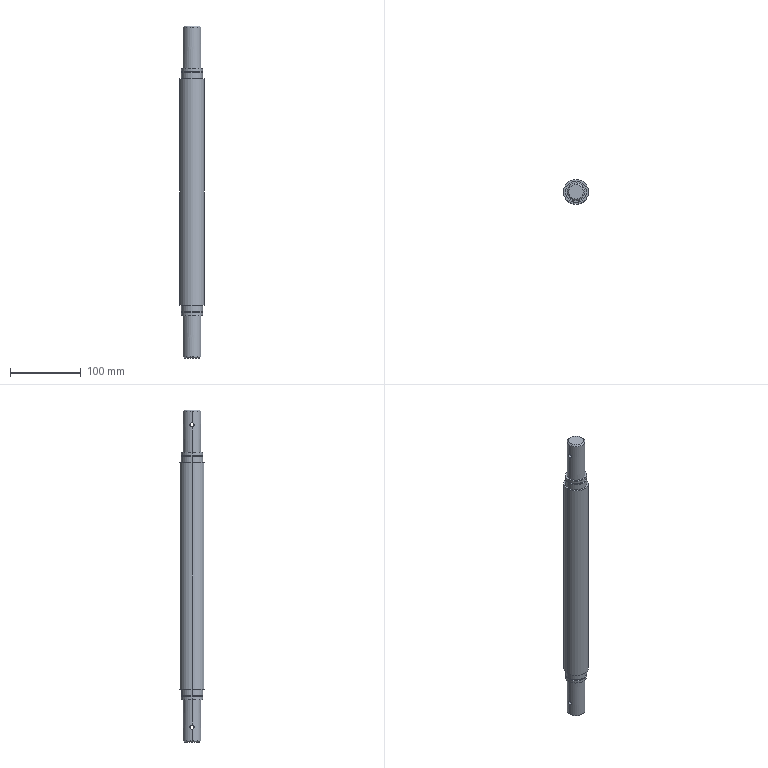Part | STEP file | Shaft 4 | 1 solid | 36 faces | box 35 x 35 x 470 mm | volume 385852 mm3 | cylinder 22 | plane 10 | cone 4 | commonest cylinder face diameters 30 x8 6 x4 25 x4 27.6 x4 35 x2
STEP:
#1=CARTESIAN_POINT('',(-17.5,0.,335.));
#2=VERTEX_POINT('',#1);
#3=CARTESIAN_POINT('',(17.5,0.,335.));
#4=VERTEX_POINT('',#3);
#5=CARTESIAN_POINT('',(0.,0.,335.));
#6=DIRECTION('',(0.,0.,-1.));
#7=DIRECTION('',(-1.,0.,0.));
#8=AXIS2_PLACEMENT_3D('',#5,#6,#7);
#9=CIRCLE('',#8,17.5);
#10=EDGE_CURVE('',#2,#4,#9,.T.);
#11=ORIENTED_EDGE('',*,*,#10,.T.);
#12=CARTESIAN_POINT('',(17.5,0.,15.));
#13=VERTEX_POINT('',#12);
#14=CARTESIAN_POINT('',(17.5,0.,350.));
#15=DIRECTION('',(0.,0.,-1.));
#16=VECTOR('',#15,1000.);
#17=LINE('',#14,#16);
#18=EDGE_CURVE('',#4,#13,#17,.T.);
#19=ORIENTED_EDGE('',*,*,#18,.T.);
#20=CARTESIAN_POINT('',(-17.5,0.,15.));
#21=VERTEX_POINT('',#20);
#22=CARTESIAN_POINT('',(0.,0.,15.));
#23=DIRECTION('',(0.,0.,1.));
#24=DIRECTION('',(-1.,0.,0.));
#25=AXIS2_PLACEMENT_3D('',#22,#23,#24);
#26=CIRCLE('',#25,17.5);
#27=EDGE_CURVE('',#13,#21,#26,.T.);
#28=ORIENTED_EDGE('',*,*,#27,.T.);
#29=CARTESIAN_POINT('',(-17.5,0.,350.));
#30=DIRECTION('',(0.,0.,-1.));
#31=VECTOR('',#30,1000.);
#32=LINE('',#29,#31);
#33=EDGE_CURVE('',#2,#21,#32,.T.);
#34=ORIENTED_EDGE('',*,*,#33,.F.);
#35=EDGE_LOOP('',(#11,#19,#28,#34));
#36=FACE_OUTER_BOUND('',#35,.T.);
#37=CARTESIAN_POINT('',(0.,0.,350.));
#38=DIRECTION('',(0.,0.,-1.));
#39=DIRECTION('',(-1.,0.,0.));
#40=AXIS2_PLACEMENT_3D('',#37,#38,#39);
#41=CYLINDRICAL_SURFACE('',#40,17.5);
#42=ADVANCED_FACE('',(#36),#41,.T.);
#43=CARTESIAN_POINT('',(15.,0.,15.));
#44=VERTEX_POINT('',#43);
#45=CARTESIAN_POINT('',(-15.,0.,15.));
#46=VERTEX_POINT('',#45);
#47=CARTESIAN_POINT('',(0.,0.,15.));
#48=DIRECTION('',(0.,0.,1.));
#49=DIRECTION('',(-1.,0.,0.));
#50=AXIS2_PLACEMENT_3D('',#47,#48,#49);
#51=CIRCLE('',#50,15.);
#52=EDGE_CURVE('',#44,#46,#51,.T.);
#53=ORIENTED_EDGE('',*,*,#52,.F.);
#54=CARTESIAN_POINT('',(15.,0.,6.));
#55=VERTEX_POINT('',#54);
#56=CARTESIAN_POINT('',(15.,0.,15.));
#57=DIRECTION('',(0.,0.,-1.));
#58=VECTOR('',#57,1000.);
#59=LINE('',#56,#58);
#60=EDGE_CURVE('',#44,#55,#59,.T.);
#61=ORIENTED_EDGE('',*,*,#60,.T.);
#62=CARTESIAN_POINT('',(-15.,0.,6.));
#63=VERTEX_POINT('',#62);
#64=CARTESIAN_POINT('',(0.,0.,6.));
#65=DIRECTION('',(0.,0.,1.));
#66=DIRECTION('',(-1.,0.,0.));
#67=AXIS2_PLACEMENT_3D('',#64,#65,#66);
#68=CIRCLE('',#67,15.);
#69=EDGE_CURVE('',#55,#63,#68,.T.);
#70=ORIENTED_EDGE('',*,*,#69,.T.);
#71=CARTESIAN_POINT('',(-15.,0.,15.));
#72=DIRECTION('',(0.,0.,-1.));
#73=VECTOR('',#72,1000.);
#74=LINE('',#71,#73);
#75=EDGE_CURVE('',#46,#63,#74,.T.);
#76=ORIENTED_EDGE('',*,*,#75,.F.);
#77=EDGE_LOOP('',(#53,#61,#70,#76));
#78=FACE_OUTER_BOUND('',#77,.T.);
#79=CARTESIAN_POINT('',(0.,0.,15.));
#80=DIRECTION('',(0.,0.,-1.));
#81=DIRECTION('',(-1.,0.,0.));
#82=AXIS2_PLACEMENT_3D('',#79,#80,#81);
#83=CYLINDRICAL_SURFACE('',#82,15.);
#84=ADVANCED_FACE('',(#78),#83,.T.);
#85=CARTESIAN_POINT('',(-15.,0.,335.));
#86=VERTEX_POINT('',#85);
#87=CARTESIAN_POINT('',(15.,0.,335.));
#88=VERTEX_POINT('',#87);
#89=CARTESIAN_POINT('',(0.,0.,335.));
#90=DIRECTION('',(0.,0.,-1.));
#91=DIRECTION('',(1.,0.,0.));
#92=AXIS2_PLACEMENT_3D('',#89,#90,#91);
#93=CIRCLE('',#92,15.);
#94=EDGE_CURVE('',#86,#88,#93,.T.);
#95=ORIENTED_EDGE('',*,*,#94,.F.);
#96=CARTESIAN_POINT('',(-15.,0.,344.));
#97=VERTEX_POINT('',#96);
#98=CARTESIAN_POINT('',(-15.,0.,335.));
#99=DIRECTION('',(0.,0.,1.));
#100=VECTOR('',#99,1000.);
#101=LINE('',#98,#100);
#102=EDGE_CURVE('',#86,#97,#101,.T.);
#103=ORIENTED_EDGE('',*,*,#102,.T.);
#104=CARTESIAN_POINT('',(15.,0.,344.));
#105=VERTEX_POINT('',#104);
#106=CARTESIAN_POINT('',(0.,0.,344.));
#107=DIRECTION('',(0.,0.,-1.));
#108=DIRECTION('',(1.,0.,0.));
#109=AXIS2_PLACEMENT_3D('',#106,#107,#108);
#110=CIRCLE('',#109,15.);
#111=EDGE_CURVE('',#97,#105,#110,.T.);
#112=ORIENTED_EDGE('',*,*,#111,.T.);
#113=CARTESIAN_POINT('',(15.,0.,335.));
#114=DIRECTION('',(0.,0.,1.));
#115=VECTOR('',#114,1000.);
#116=LINE('',#113,#115);
#117=EDGE_CURVE('',#88,#105,#116,.T.);
#118=ORIENTED_EDGE('',*,*,#117,.F.);
#119=EDGE_LOOP('',(#95,#103,#112,#118));
#120=FACE_OUTER_BOUND('',#119,.T.);
#121=CARTESIAN_POINT('',(0.,0.,335.));
#122=DIRECTION('',(0.,0.,1.));
#123=DIRECTION('',(1.,0.,0.));
#124=AXIS2_PLACEMENT_3D('',#121,#122,#123);
#125=CYLINDRICAL_SURFACE('',#124,15.);
#126=ADVANCED_FACE('',(#120),#125,.T.);
#127=CARTESIAN_POINT('',(-13.8,0.,6.));
#128=VERTEX_POINT('',#127);
#129=CARTESIAN_POINT('',(13.8,0.,6.));
#130=VERTEX_POINT('',#129);
#131=CARTESIAN_POINT('',(0.,0.,6.));
#132=DIRECTION('',(0.,0.,-1.));
#133=DIRECTION('',(-1.,0.,0.));
#134=AXIS2_PLACEMENT_3D('',#131,#132,#133);
#135=CIRCLE('',#134,13.8);
#136=EDGE_CURVE('',#128,#130,#135,.T.);
#137=ORIENTED_EDGE('',*,*,#136,.T.);
#138=CARTESIAN_POINT('',(13.8,0.,4.));
#139=VERTEX_POINT('',#138);
#140=CARTESIAN_POINT('',(13.8,0.,0.));
#141=DIRECTION('',(0.,0.,-1.));
#142=VECTOR('',#141,1000.);
#143=LINE('',#140,#142);
#144=EDGE_CURVE('',#130,#139,#143,.T.);
#145=ORIENTED_EDGE('',*,*,#144,.T.);
#146=CARTESIAN_POINT('',(-13.8,0.,4.));
#147=VERTEX_POINT('',#146);
#148=CARTESIAN_POINT('',(0.,0.,4.));
#149=DIRECTION('',(0.,0.,1.));
#150=DIRECTION('',(-1.,0.,0.));
#151=AXIS2_PLACEMENT_3D('',#148,#149,#150);
#152=CIRCLE('',#151,13.8);
#153=EDGE_CURVE('',#139,#147,#152,.T.);
#154=ORIENTED_EDGE('',*,*,#153,.T.);
#155=CARTESIAN_POINT('',(-13.8,0.,0.));
#156=DIRECTION('',(0.,0.,-1.));
#157=VECTOR('',#156,1000.);
#158=LINE('',#155,#157);
#159=EDGE_CURVE('',#128,#147,#158,.T.);
#160=ORIENTED_EDGE('',*,*,#159,.F.);
#161=EDGE_LOOP('',(#137,#145,#154,#160));
#162=FACE_OUTER_BOUND('',#161,.T.);
#163=CARTESIAN_POINT('',(0.,0.,0.));
#164=DIRECTION('',(0.,0.,-1.));
#165=DIRECTION('',(-1.,0.,0.));
#166=AXIS2_PLACEMENT_3D('',#163,#164,#165);
#167=CYLINDRICAL_SURFACE('',#166,13.8);
#168=ADVANCED_FACE('',(#162),#167,.T.);
#169=CARTESIAN_POINT('',(-13.8,0.,346.));
#170=VERTEX_POINT('',#169);
#171=CARTESIAN_POINT('',(13.8,0.,346.));
#172=VERTEX_POINT('',#171);
#173=CARTESIAN_POINT('',(0.,0.,346.));
#174=DIRECTION('',(0.,0.,-1.));
#175=DIRECTION('',(-1.,0.,0.));
#176=AXIS2_PLACEMENT_3D('',#173,#174,#175);
#177=CIRCLE('',#176,13.8);
#178=EDGE_CURVE('',#170,#172,#177,.T.);
#179=ORIENTED_EDGE('',*,*,#178,.T.);
#180=CARTESIAN_POINT('',(13.8,0.,344.));
#181=VERTEX_POINT('',#180);
#182=CARTESIAN_POINT('',(13.8,0.,0.));
#183=DIRECTION('',(0.,0.,-1.));
#184=VECTOR('',#183,1000.);
#185=LINE('',#182,#184);
#186=EDGE_CURVE('',#172,#181,#185,.T.);
#187=ORIENTED_EDGE('',*,*,#186,.T.);
#188=CARTESIAN_POINT('',(-13.8,0.,344.));
#189=VERTEX_POINT('',#188);
#190=CARTESIAN_POINT('',(0.,0.,344.));
#191=DIRECTION('',(0.,0.,1.));
#192=DIRECTION('',(-1.,0.,0.));
#193=AXIS2_PLACEMENT_3D('',#190,#191,#192);
#194=CIRCLE('',#193,13.8);
#195=EDGE_CURVE('',#181,#189,#194,.T.);
#196=ORIENTED_EDGE('',*,*,#195,.T.);
#197=CARTESIAN_POINT('',(-13.8,0.,0.));
#198=DIRECTION('',(0.,0.,-1.));
#199=VECTOR('',#198,1000.);
#200=LINE('',#197,#199);
#201=EDGE_CURVE('',#170,#189,#200,.T.);
#202=ORIENTED_EDGE('',*,*,#201,.F.);
#203=EDGE_LOOP('',(#179,#187,#196,#202));
#204=FACE_OUTER_BOUND('',#203,.T.);
#205=CARTESIAN_POINT('',(0.,0.,0.));
#206=DIRECTION('',(0.,0.,-1.));
#207=DIRECTION('',(-1.,0.,0.));
#208=AXIS2_PLACEMENT_3D('',#205,#206,#207);
#209=CYLINDRICAL_SURFACE('',#208,13.8);
#210=ADVANCED_FACE('',(#204),#209,.T.);
#211=CARTESIAN_POINT('',(-15.,0.,4.));
#212=VERTEX_POINT('',#211);
#213=CARTESIAN_POINT('',(15.,0.,4.));
#214=VERTEX_POINT('',#213);
#215=CARTESIAN_POINT('',(0.,0.,4.));
#216=DIRECTION('',(0.,0.,-1.));
#217=DIRECTION('',(-1.,0.,0.));
#218=AXIS2_PLACEMENT_3D('',#215,#216,#217);
#219=CIRCLE('',#218,15.);
#220=EDGE_CURVE('',#212,#214,#219,.T.);
#221=ORIENTED_EDGE('',*,*,#220,.T.);
#222=CARTESIAN_POINT('',(15.,0.,0.));
#223=VERTEX_POINT('',#222);
#224=CARTESIAN_POINT('',(15.,0.,15.));
#225=DIRECTION('',(0.,0.,-1.));
#226=VECTOR('',#225,1000.);
#227=LINE('',#224,#226);
#228=EDGE_CURVE('',#214,#223,#227,.T.);
#229=ORIENTED_EDGE('',*,*,#228,.T.);
#230=CARTESIAN_POINT('',(-15.,0.,0.));
#231=VERTEX_POINT('',#230);
#232=CARTESIAN_POINT('',(0.,0.,0.));
#233=DIRECTION('',(0.,0.,1.));
#234=DIRECTION('',(-1.,0.,0.));
#235=AXIS2_PLACEMENT_3D('',#232,#233,#234);
#236=CIRCLE('',#235,15.);
#237=EDGE_CURVE('',#223,#231,#236,.T.);
#238=ORIENTED_EDGE('',*,*,#237,.T.);
#239=CARTESIAN_POINT('',(-15.,0.,15.));
#240=DIRECTION('',(0.,0.,-1.));
#241=VECTOR('',#240,1000.);
#242=LINE('',#239,#241);
#243=EDGE_CURVE('',#212,#231,#242,.T.);
#244=ORIENTED_EDGE('',*,*,#243,.F.);
#245=EDGE_LOOP('',(#221,#229,#238,#244));
#246=FACE_OUTER_BOUND('',#245,.T.);
#247=CARTESIAN_POINT('',(0.,0.,15.));
#248=DIRECTION('',(0.,0.,-1.));
#249=DIRECTION('',(-1.,0.,0.));
#250=AXIS2_PLACEMENT_3D('',#247,#248,#249);
#251=CYLINDRICAL_SURFACE('',#250,15.);
#252=ADVANCED_FACE('',(#246),#251,.T.);
#253=CARTESIAN_POINT('',(15.,0.,346.));
#254=VERTEX_POINT('',#253);
#255=CARTESIAN_POINT('',(-15.,0.,346.));
#256=VERTEX_POINT('',#255);
#257=CARTESIAN_POINT('',(0.,0.,346.));
#258=DIRECTION('',(0.,0.,1.));
#259=DIRECTION('',(1.,0.,0.));
#260=AXIS2_PLACEMENT_3D('',#257,#258,#259);
#261=CIRCLE('',#260,15.);
#262=EDGE_CURVE('',#254,#256,#261,.T.);
#263=ORIENTED_EDGE('',*,*,#262,.T.);
#264=CARTESIAN_POINT('',(-15.,0.,350.));
#265=VERTEX_POINT('',#264);
#266=CARTESIAN_POINT('',(-15.,0.,335.));
#267=DIRECTION('',(0.,0.,1.));
#268=VECTOR('',#267,1000.);
#269=LINE('',#266,#268);
#270=EDGE_CURVE('',#256,#265,#269,.T.);
#271=ORIENTED_EDGE('',*,*,#270,.T.);
#272=CARTESIAN_POINT('',(15.,0.,350.));
#273=VERTEX_POINT('',#272);
#274=CARTESIAN_POINT('',(0.,0.,350.));
#275=DIRECTION('',(0.,0.,-1.));
#276=DIRECTION('',(1.,0.,0.));
#277=AXIS2_PLACEMENT_3D('',#274,#275,#276);
#278=CIRCLE('',#277,15.);
#279=EDGE_CURVE('',#265,#273,#278,.T.);
#280=ORIENTED_EDGE('',*,*,#279,.T.);
#281=CARTESIAN_POINT('',(15.,0.,335.));
#282=DIRECTION('',(0.,0.,1.));
#283=VECTOR('',#282,1000.);
#284=LINE('',#281,#283);
#285=EDGE_CURVE('',#254,#273,#284,.T.);
#286=ORIENTED_EDGE('',*,*,#285,.F.);
#287=EDGE_LOOP('',(#263,#271,#280,#286));
#288=FACE_OUTER_BOUND('',#287,.T.);
#289=CARTESIAN_POINT('',(0.,0.,335.));
#290=DIRECTION('',(0.,0.,1.));
#291=DIRECTION('',(1.,0.,0.));
#292=AXIS2_PLACEMENT_3D('',#289,#290,#291);
#293=CYLINDRICAL_SURFACE('',#292,15.);
#294=ADVANCED_FACE('',(#288),#293,.T.);
#295=CARTESIAN_POINT('',(0.,12.5,-58.));
#296=VERTEX_POINT('',#295);
#297=CARTESIAN_POINT('',(-12.5,0.,-58.));
#298=VERTEX_POINT('',#297);
#299=CARTESIAN_POINT('',(0.,0.,-58.));
#300=DIRECTION('',(0.,0.,1.));
#301=DIRECTION('',(1.,0.,0.));
#302=AXIS2_PLACEMENT_3D('',#299,#300,#301);
#303=CIRCLE('',#302,12.5);
#304=EDGE_CURVE('',#296,#298,#303,.T.);
#305=ORIENTED_EDGE('',*,*,#304,.T.);
#306=CARTESIAN_POINT('',(-12.5,0.,-42.));
#307=VERTEX_POINT('',#306);
#308=CARTESIAN_POINT('',(-12.5,0.,-60.));
#309=DIRECTION('',(0.,0.,1.));
#310=VECTOR('',#309,1000.);
#311=LINE('',#308,#310);
#312=EDGE_CURVE('',#298,#307,#311,.T.);
#313=ORIENTED_EDGE('',*,*,#312,.T.);
#314=CARTESIAN_POINT('',(-12.5,0.,-36.));
#315=VERTEX_POINT('',#314);
#316=CARTESIAN_POINT('',(-12.5,0.,-42.));
#317=CARTESIAN_POINT('',(-12.5,0.1989,-42.));
#318=CARTESIAN_POINT('',(-12.495,0.3944,-41.98));
#319=CARTESIAN_POINT('',(-12.477,0.7788,-41.904));
#320=CARTESIAN_POINT('',(-12.464,0.9697,-41.846));
#321=CARTESIAN_POINT('',(-12.43,1.333,-41.695));
#322=CARTESIAN_POINT('',(-12.41,1.505,-41.603));
#323=CARTESIAN_POINT('',(-12.366,1.83,-41.385));
#324=CARTESIAN_POINT('',(-12.342,1.984,-41.259));
#325=CARTESIAN_POINT('',(-12.295,2.259,-40.983));
#326=CARTESIAN_POINT('',(-12.271,2.383,-40.833));
#327=CARTESIAN_POINT('',(-12.227,2.602,-40.505));
#328=CARTESIAN_POINT('',(-12.206,2.695,-40.332));
#329=CARTESIAN_POINT('',(-12.172,2.845,-39.971));
#330=CARTESIAN_POINT('',(-12.158,2.903,-39.782));
#331=CARTESIAN_POINT('',(-12.14,2.981,-39.394));
#332=CARTESIAN_POINT('',(-12.135,3.,-39.199));
#333=CARTESIAN_POINT('',(-12.135,3.,-38.806));
#334=CARTESIAN_POINT('',(-12.14,2.981,-38.607));
#335=CARTESIAN_POINT('',(-12.158,2.904,-38.221));
#336=CARTESIAN_POINT('',(-12.172,2.847,-38.034));
#337=CARTESIAN_POINT('',(-12.206,2.696,-37.67));
#338=CARTESIAN_POINT('',(-12.227,2.603,-37.495));
#339=CARTESIAN_POINT('',(-12.271,2.386,-37.171));
#340=CARTESIAN_POINT('',(-12.295,2.261,-37.019));
#341=CARTESIAN_POINT('',(-12.342,1.983,-36.741));
#342=CARTESIAN_POINT('',(-12.366,1.833,-36.617));
#343=CARTESIAN_POINT('',(-12.41,1.509,-36.4));
#344=CARTESIAN_POINT('',(-12.43,1.333,-36.305));
#345=CARTESIAN_POINT('',(-12.464,0.9711,-36.155));
#346=CARTESIAN_POINT('',(-12.477,0.7841,-36.098));
#347=CARTESIAN_POINT('',(-12.495,0.3981,-36.02));
#348=CARTESIAN_POINT('',(-12.5,0.1989,-36.));
#349=CARTESIAN_POINT('',(-12.5,0.,-36.));
#350=B_SPLINE_CURVE_WITH_KNOTS('',3,(#316,#317,#318,#319,#320,#321,#322,#323,#324,#325,#326,#327,#328,#329,#330,#331,#332,#333,#334,#335,#336,#337,#338,#339,#340,#341,#342,#343,#344,#345,#346,#347,#348,#349),.UNSPECIFIED.,.F.,.F.,(4,2,2,2,2,2,2,2,2,2,2,2,2,2,2,2,4),(0.009411,0.009999,0.01059,0.01118,0.01176,0.01235,0.01294,0.01353,0.01412,0.0147,0.01529,0.01588,0.01647,0.01706,0.01765,0.01823,0.01882),.UNSPECIFIED.);
#351=EDGE_CURVE('',#307,#315,#350,.T.);
#352=ORIENTED_EDGE('',*,*,#351,.T.);
#353=CARTESIAN_POINT('',(-12.5,0.,0.));
#354=VERTEX_POINT('',#353);
#355=CARTESIAN_POINT('',(-12.5,0.,-60.));
#356=DIRECTION('',(0.,0.,1.));
#357=VECTOR('',#356,1000.);
#358=LINE('',#355,#357);
#359=EDGE_CURVE('',#315,#354,#358,.T.);
#360=ORIENTED_EDGE('',*,*,#359,.T.);
#361=CARTESIAN_POINT('',(12.5,0.,0.));
#362=VERTEX_POINT('',#361);
#363=CARTESIAN_POINT('',(0.,0.,0.));
#364=DIRECTION('',(0.,0.,-1.));
#365=DIRECTION('',(1.,0.,0.));
#366=AXIS2_PLACEMENT_3D('',#363,#364,#365);
#367=CIRCLE('',#366,12.5);
#368=EDGE_CURVE('',#354,#362,#367,.T.);
#369=ORIENTED_EDGE('',*,*,#368,.T.);
#370=CARTESIAN_POINT('',(12.5,0.,-36.));
#371=VERTEX_POINT('',#370);
#372=CARTESIAN_POINT('',(12.5,0.,-60.));
#373=DIRECTION('',(0.,0.,1.));
#374=VECTOR('',#373,1000.);
#375=LINE('',#372,#374);
#376=EDGE_CURVE('',#371,#362,#375,.T.);
#377=ORIENTED_EDGE('',*,*,#376,.F.);
#378=CARTESIAN_POINT('',(12.5,0.,-42.));
#379=VERTEX_POINT('',#378);
#380=CARTESIAN_POINT('',(12.5,0.,-36.));
#381=CARTESIAN_POINT('',(12.5,0.1989,-36.));
#382=CARTESIAN_POINT('',(12.495,0.3944,-36.02));
#383=CARTESIAN_POINT('',(12.477,0.7788,-36.096));
#384=CARTESIAN_POINT('',(12.464,0.9697,-36.154));
#385=CARTESIAN_POINT('',(12.43,1.333,-36.305));
#386=CARTESIAN_POINT('',(12.41,1.505,-36.397));
#387=CARTESIAN_POINT('',(12.366,1.83,-36.615));
#388=CARTESIAN_POINT('',(12.342,1.984,-36.741));
#389=CARTESIAN_POINT('',(12.295,2.259,-37.017));
#390=CARTESIAN_POINT('',(12.271,2.383,-37.167));
#391=CARTESIAN_POINT('',(12.227,2.602,-37.495));
#392=CARTESIAN_POINT('',(12.206,2.695,-37.668));
#393=CARTESIAN_POINT('',(12.172,2.845,-38.029));
#394=CARTESIAN_POINT('',(12.158,2.903,-38.218));
#395=CARTESIAN_POINT('',(12.14,2.981,-38.606));
#396=CARTESIAN_POINT('',(12.135,3.,-38.801));
#397=CARTESIAN_POINT('',(12.135,3.,-39.194));
#398=CARTESIAN_POINT('',(12.14,2.981,-39.393));
#399=CARTESIAN_POINT('',(12.158,2.904,-39.779));
#400=CARTESIAN_POINT('',(12.172,2.847,-39.966));
#401=CARTESIAN_POINT('',(12.206,2.696,-40.33));
#402=CARTESIAN_POINT('',(12.227,2.603,-40.505));
#403=CARTESIAN_POINT('',(12.271,2.386,-40.829));
#404=CARTESIAN_POINT('',(12.295,2.261,-40.981));
#405=CARTESIAN_POINT('',(12.342,1.983,-41.259));
#406=CARTESIAN_POINT('',(12.366,1.833,-41.383));
#407=CARTESIAN_POINT('',(12.41,1.509,-41.6));
#408=CARTESIAN_POINT('',(12.43,1.333,-41.695));
#409=CARTESIAN_POINT('',(12.464,0.9711,-41.845));
#410=CARTESIAN_POINT('',(12.477,0.7841,-41.902));
#411=CARTESIAN_POINT('',(12.495,0.3981,-41.98));
#412=CARTESIAN_POINT('',(12.5,0.1989,-42.));
#413=CARTESIAN_POINT('',(12.5,0.,-42.));
#414=B_SPLINE_CURVE_WITH_KNOTS('',3,(#380,#381,#382,#383,#384,#385,#386,#387,#388,#389,#390,#391,#392,#393,#394,#395,#396,#397,#398,#399,#400,#401,#402,#403,#404,#405,#406,#407,#408,#409,#410,#411,#412,#413),.UNSPECIFIED.,.F.,.F.,(4,2,2,2,2,2,2,2,2,2,2,2,2,2,2,2,4),(0.009411,0.009999,0.01059,0.01118,0.01176,0.01235,0.01294,0.01353,0.01412,0.0147,0.01529,0.01588,0.01647,0.01706,0.01765,0.01823,0.01882),.UNSPECIFIED.);
#415=EDGE_CURVE('',#371,#379,#414,.T.);
#416=ORIENTED_EDGE('',*,*,#415,.T.);
#417=CARTESIAN_POINT('',(12.5,0.,-58.));
#418=VERTEX_POINT('',#417);
#419=CARTESIAN_POINT('',(12.5,0.,-60.));
#420=DIRECTION('',(0.,0.,1.));
#421=VECTOR('',#420,1000.);
#422=LINE('',#419,#421);
#423=EDGE_CURVE('',#418,#379,#422,.T.);
#424=ORIENTED_EDGE('',*,*,#423,.F.);
#425=CARTESIAN_POINT('',(0.,0.,-58.));
#426=DIRECTION('',(0.,0.,1.));
#427=DIRECTION('',(1.,0.,0.));
#428=AXIS2_PLACEMENT_3D('',#425,#426,#427);
#429=CIRCLE('',#428,12.5);
#430=EDGE_CURVE('',#418,#296,#429,.T.);
#431=ORIENTED_EDGE('',*,*,#430,.T.);
#432=EDGE_LOOP('',(#305,#313,#352,#360,#369,#377,#416,#424,#431));
#433=FACE_OUTER_BOUND('',#432,.T.);
#434=CARTESIAN_POINT('',(0.,0.,-60.));
#435=DIRECTION('',(0.,0.,1.));
#436=DIRECTION('',(1.,0.,0.));
#437=AXIS2_PLACEMENT_3D('',#434,#435,#436);
#438=CYLINDRICAL_SURFACE('',#437,12.5);
#439=ADVANCED_FACE('',(#433),#438,.T.);
#440=CARTESIAN_POINT('',(0.,12.5,408.));
#441=VERTEX_POINT('',#440);
#442=CARTESIAN_POINT('',(12.5,0.,408.));
#443=VERTEX_POINT('',#442);
#444=CARTESIAN_POINT('',(0.,0.,408.));
#445=DIRECTION('',(0.,0.,-1.));
#446=DIRECTION('',(-1.,0.,0.));
#447=AXIS2_PLACEMENT_3D('',#444,#445,#446);
#448=CIRCLE('',#447,12.5);
#449=EDGE_CURVE('',#441,#443,#448,.T.);
#450=ORIENTED_EDGE('',*,*,#449,.T.);
#451=CARTESIAN_POINT('',(12.5,0.,392.));
#452=VERTEX_POINT('',#451);
#453=CARTESIAN_POINT('',(12.5,0.,410.));
#454=DIRECTION('',(0.,0.,-1.));
#455=VECTOR('',#454,1000.);
#456=LINE('',#453,#455);
#457=EDGE_CURVE('',#443,#452,#456,.T.);
#458=ORIENTED_EDGE('',*,*,#457,.T.);
#459=CARTESIAN_POINT('',(12.5,0.,386.));
#460=VERTEX_POINT('',#459);
#461=CARTESIAN_POINT('',(12.5,0.,392.));
#462=CARTESIAN_POINT('',(12.5,0.1989,392.));
#463=CARTESIAN_POINT('',(12.495,0.3944,391.98));
#464=CARTESIAN_POINT('',(12.477,0.7788,391.904));
#465=CARTESIAN_POINT('',(12.464,0.9697,391.846));
#466=CARTESIAN_POINT('',(12.43,1.333,391.695));
#467=CARTESIAN_POINT('',(12.41,1.505,391.603));
#468=CARTESIAN_POINT('',(12.366,1.83,391.385));
#469=CARTESIAN_POINT('',(12.342,1.984,391.259));
#470=CARTESIAN_POINT('',(12.295,2.259,390.983));
#471=CARTESIAN_POINT('',(12.271,2.383,390.833));
#472=CARTESIAN_POINT('',(12.227,2.602,390.505));
#473=CARTESIAN_POINT('',(12.206,2.695,390.332));
#474=CARTESIAN_POINT('',(12.172,2.845,389.971));
#475=CARTESIAN_POINT('',(12.158,2.903,389.782));
#476=CARTESIAN_POINT('',(12.14,2.981,389.394));
#477=CARTESIAN_POINT('',(12.135,3.,389.199));
#478=CARTESIAN_POINT('',(12.135,3.,388.806));
#479=CARTESIAN_POINT('',(12.14,2.981,388.607));
#480=CARTESIAN_POINT('',(12.158,2.904,388.221));
#481=CARTESIAN_POINT('',(12.172,2.847,388.034));
#482=CARTESIAN_POINT('',(12.206,2.696,387.67));
#483=CARTESIAN_POINT('',(12.227,2.603,387.495));
#484=CARTESIAN_POINT('',(12.271,2.386,387.171));
#485=CARTESIAN_POINT('',(12.295,2.261,387.019));
#486=CARTESIAN_POINT('',(12.342,1.983,386.741));
#487=CARTESIAN_POINT('',(12.366,1.833,386.617));
#488=CARTESIAN_POINT('',(12.41,1.509,386.4));
#489=CARTESIAN_POINT('',(12.43,1.333,386.305));
#490=CARTESIAN_POINT('',(12.464,0.9711,386.155));
#491=CARTESIAN_POINT('',(12.477,0.7841,386.098));
#492=CARTESIAN_POINT('',(12.495,0.3981,386.02));
#493=CARTESIAN_POINT('',(12.5,0.1989,386.));
#494=CARTESIAN_POINT('',(12.5,0.,386.));
#495=B_SPLINE_CURVE_WITH_KNOTS('',3,(#461,#462,#463,#464,#465,#466,#467,#468,#469,#470,#471,#472,#473,#474,#475,#476,#477,#478,#479,#480,#481,#482,#483,#484,#485,#486,#487,#488,#489,#490,#491,#492,#493,#494),.UNSPECIFIED.,.F.,.F.,(4,2,2,2,2,2,2,2,2,2,2,2,2,2,2,2,4),(0.,0.0005882,0.001176,0.001765,0.002353,0.002941,0.003529,0.004117,0.004706,0.005294,0.005882,0.00647,0.007058,0.007646,0.008235,0.008823,0.009411),.UNSPECIFIED.);
#496=EDGE_CURVE('',#452,#460,#495,.T.);
#497=ORIENTED_EDGE('',*,*,#496,.T.);
#498=CARTESIAN_POINT('',(12.5,0.,350.));
#499=VERTEX_POINT('',#498);
#500=CARTESIAN_POINT('',(12.5,0.,410.));
#501=DIRECTION('',(0.,0.,-1.));
#502=VECTOR('',#501,1000.);
#503=LINE('',#500,#502);
#504=EDGE_CURVE('',#460,#499,#503,.T.);
#505=ORIENTED_EDGE('',*,*,#504,.T.);
#506=CARTESIAN_POINT('',(-12.5,0.,350.));
#507=VERTEX_POINT('',#506);
#508=CARTESIAN_POINT('',(0.,0.,350.));
#509=DIRECTION('',(0.,0.,-1.));
#510=DIRECTION('',(-1.,0.,0.));
#511=AXIS2_PLACEMENT_3D('',#508,#509,#510);
#512=CIRCLE('',#511,12.5);
#513=EDGE_CURVE('',#507,#499,#512,.T.);
#514=ORIENTED_EDGE('',*,*,#513,.F.);
#515=CARTESIAN_POINT('',(-12.5,0.,386.));
#516=VERTEX_POINT('',#515);
#517=CARTESIAN_POINT('',(-12.5,0.,410.));
#518=DIRECTION('',(0.,0.,-1.));
#519=VECTOR('',#518,1000.);
#520=LINE('',#517,#519);
#521=EDGE_CURVE('',#516,#507,#520,.T.);
#522=ORIENTED_EDGE('',*,*,#521,.F.);
#523=CARTESIAN_POINT('',(-12.5,0.,392.));
#524=VERTEX_POINT('',#523);
#525=CARTESIAN_POINT('',(-12.5,0.,386.));
#526=CARTESIAN_POINT('',(-12.5,0.1989,386.));
#527=CARTESIAN_POINT('',(-12.495,0.3944,386.02));
#528=CARTESIAN_POINT('',(-12.477,0.7788,386.096));
#529=CARTESIAN_POINT('',(-12.464,0.9697,386.154));
#530=CARTESIAN_POINT('',(-12.43,1.333,386.305));
#531=CARTESIAN_POINT('',(-12.41,1.505,386.397));
#532=CARTESIAN_POINT('',(-12.366,1.83,386.615));
#533=CARTESIAN_POINT('',(-12.342,1.984,386.741));
#534=CARTESIAN_POINT('',(-12.295,2.259,387.017));
#535=CARTESIAN_POINT('',(-12.271,2.383,387.167));
#536=CARTESIAN_POINT('',(-12.227,2.602,387.495));
#537=CARTESIAN_POINT('',(-12.206,2.695,387.668));
#538=CARTESIAN_POINT('',(-12.172,2.845,388.029));
#539=CARTESIAN_POINT('',(-12.158,2.903,388.218));
#540=CARTESIAN_POINT('',(-12.14,2.981,388.606));
#541=CARTESIAN_POINT('',(-12.135,3.,388.801));
#542=CARTESIAN_POINT('',(-12.135,3.,389.194));
#543=CARTESIAN_POINT('',(-12.14,2.981,389.393));
#544=CARTESIAN_POINT('',(-12.158,2.904,389.779));
#545=CARTESIAN_POINT('',(-12.172,2.847,389.966));
#546=CARTESIAN_POINT('',(-12.206,2.696,390.33));
#547=CARTESIAN_POINT('',(-12.227,2.603,390.505));
#548=CARTESIAN_POINT('',(-12.271,2.386,390.829));
#549=CARTESIAN_POINT('',(-12.295,2.261,390.981));
#550=CARTESIAN_POINT('',(-12.342,1.983,391.259));
#551=CARTESIAN_POINT('',(-12.366,1.833,391.383));
#552=CARTESIAN_POINT('',(-12.41,1.509,391.6));
#553=CARTESIAN_POINT('',(-12.43,1.333,391.695));
#554=CARTESIAN_POINT('',(-12.464,0.9711,391.845));
#555=CARTESIAN_POINT('',(-12.477,0.7841,391.902));
#556=CARTESIAN_POINT('',(-12.495,0.3981,391.98));
#557=CARTESIAN_POINT('',(-12.5,0.1989,392.));
#558=CARTESIAN_POINT('',(-12.5,0.,392.));
#559=B_SPLINE_CURVE_WITH_KNOTS('',3,(#525,#526,#527,#528,#529,#530,#531,#532,#533,#534,#535,#536,#537,#538,#539,#540,#541,#542,#543,#544,#545,#546,#547,#548,#549,#550,#551,#552,#553,#554,#555,#556,#557,#558),.UNSPECIFIED.,.F.,.F.,(4,2,2,2,2,2,2,2,2,2,2,2,2,2,2,2,4),(0.,0.0005882,0.001176,0.001765,0.002353,0.002941,0.003529,0.004117,0.004706,0.005294,0.005882,0.00647,0.007058,0.007646,0.008235,0.008823,0.009411),.UNSPECIFIED.);
#560=EDGE_CURVE('',#516,#524,#559,.T.);
#561=ORIENTED_EDGE('',*,*,#560,.T.);
#562=CARTESIAN_POINT('',(-12.5,0.,408.));
#563=VERTEX_POINT('',#562);
#564=CARTESIAN_POINT('',(-12.5,0.,410.));
#565=DIRECTION('',(0.,0.,-1.));
#566=VECTOR('',#565,1000.);
#567=LINE('',#564,#566);
#568=EDGE_CURVE('',#563,#524,#567,.T.);
#569=ORIENTED_EDGE('',*,*,#568,.F.);
#570=CARTESIAN_POINT('',(0.,0.,408.));
#571=DIRECTION('',(0.,0.,-1.));
#572=DIRECTION('',(-1.,0.,0.));
#573=AXIS2_PLACEMENT_3D('',#570,#571,#572);
#574=CIRCLE('',#573,12.5);
#575=EDGE_CURVE('',#563,#441,#574,.T.);
#576=ORIENTED_EDGE('',*,*,#575,.T.);
#577=EDGE_LOOP('',(#450,#458,#497,#505,#514,#522,#561,#569,#576));
#578=FACE_OUTER_BOUND('',#577,.T.);
#579=CARTESIAN_POINT('',(0.,0.,410.));
#580=DIRECTION('',(0.,0.,-1.));
#581=DIRECTION('',(-1.,0.,0.));
#582=AXIS2_PLACEMENT_3D('',#579,#580,#581);
#583=CYLINDRICAL_SURFACE('',#582,12.5);
#584=ADVANCED_FACE('',(#578),#583,.T.);
#585=CARTESIAN_POINT('',(-12.5,0.,-36.));
#586=CARTESIAN_POINT('',(-12.5,-0.1989,-36.));
#587=CARTESIAN_POINT('',(-12.495,-0.3944,-36.02));
#588=CARTESIAN_POINT('',(-12.477,-0.7788,-36.096));
#589=CARTESIAN_POINT('',(-12.464,-0.9697,-36.154));
#590=CARTESIAN_POINT('',(-12.43,-1.333,-36.305));
#591=CARTESIAN_POINT('',(-12.41,-1.505,-36.397));
#592=CARTESIAN_POINT('',(-12.366,-1.83,-36.615));
#593=CARTESIAN_POINT('',(-12.342,-1.984,-36.741));
#594=CARTESIAN_POINT('',(-12.295,-2.259,-37.017));
#595=CARTESIAN_POINT('',(-12.271,-2.383,-37.167));
#596=CARTESIAN_POINT('',(-12.227,-2.602,-37.495));
#597=CARTESIAN_POINT('',(-12.206,-2.695,-37.668));
#598=CARTESIAN_POINT('',(-12.172,-2.845,-38.029));
#599=CARTESIAN_POINT('',(-12.158,-2.903,-38.218));
#600=CARTESIAN_POINT('',(-12.14,-2.981,-38.606));
#601=CARTESIAN_POINT('',(-12.135,-3.,-38.801));
#602=CARTESIAN_POINT('',(-12.135,-3.,-39.194));
#603=CARTESIAN_POINT('',(-12.14,-2.981,-39.393));
#604=CARTESIAN_POINT('',(-12.158,-2.904,-39.779));
#605=CARTESIAN_POINT('',(-12.172,-2.847,-39.966));
#606=CARTESIAN_POINT('',(-12.206,-2.696,-40.33));
#607=CARTESIAN_POINT('',(-12.227,-2.603,-40.505));
#608=CARTESIAN_POINT('',(-12.271,-2.386,-40.829));
#609=CARTESIAN_POINT('',(-12.295,-2.261,-40.981));
#610=CARTESIAN_POINT('',(-12.342,-1.983,-41.259));
#611=CARTESIAN_POINT('',(-12.366,-1.833,-41.383));
#612=CARTESIAN_POINT('',(-12.41,-1.509,-41.6));
#613=CARTESIAN_POINT('',(-12.43,-1.333,-41.695));
#614=CARTESIAN_POINT('',(-12.464,-0.9711,-41.845));
#615=CARTESIAN_POINT('',(-12.477,-0.7841,-41.902));
#616=CARTESIAN_POINT('',(-12.495,-0.3981,-41.98));
#617=CARTESIAN_POINT('',(-12.5,-0.1989,-42.));
#618=CARTESIAN_POINT('',(-12.5,0.,-42.));
#619=B_SPLINE_CURVE_WITH_KNOTS('',3,(#585,#586,#587,#588,#589,#590,#591,#592,#593,#594,#595,#596,#597,#598,#599,#600,#601,#602,#603,#604,#605,#606,#607,#608,#609,#610,#611,#612,#613,#614,#615,#616,#617,#618),.UNSPECIFIED.,.F.,.F.,(4,2,2,2,2,2,2,2,2,2,2,2,2,2,2,2,4),(0.,0.0005882,0.001176,0.001765,0.002353,0.002941,0.003529,0.004117,0.004706,0.005294,0.005882,0.00647,0.007058,0.007646,0.008235,0.008823,0.009411),.UNSPECIFIED.);
#620=EDGE_CURVE('',#315,#307,#619,.T.);
#621=ORIENTED_EDGE('',*,*,#620,.F.);
#622=CARTESIAN_POINT('',(-15.,0.,-36.));
#623=DIRECTION('',(1.,0.,0.));
#624=VECTOR('',#623,1000.);
#625=LINE('',#622,#624);
#626=EDGE_CURVE('',#315,#371,#625,.T.);
#627=ORIENTED_EDGE('',*,*,#626,.T.);
#628=CARTESIAN_POINT('',(12.5,0.,-42.));
#629=CARTESIAN_POINT('',(12.5,-0.1989,-42.));
#630=CARTESIAN_POINT('',(12.495,-0.3944,-41.98));
#631=CARTESIAN_POINT('',(12.477,-0.7788,-41.904));
#632=CARTESIAN_POINT('',(12.464,-0.9697,-41.846));
#633=CARTESIAN_POINT('',(12.43,-1.333,-41.695));
#634=CARTESIAN_POINT('',(12.41,-1.505,-41.603));
#635=CARTESIAN_POINT('',(12.366,-1.83,-41.385));
#636=CARTESIAN_POINT('',(12.342,-1.984,-41.259));
#637=CARTESIAN_POINT('',(12.295,-2.259,-40.983));
#638=CARTESIAN_POINT('',(12.271,-2.383,-40.833));
#639=CARTESIAN_POINT('',(12.227,-2.602,-40.505));
#640=CARTESIAN_POINT('',(12.206,-2.695,-40.332));
#641=CARTESIAN_POINT('',(12.172,-2.845,-39.971));
#642=CARTESIAN_POINT('',(12.158,-2.903,-39.782));
#643=CARTESIAN_POINT('',(12.14,-2.981,-39.394));
#644=CARTESIAN_POINT('',(12.135,-3.,-39.199));
#645=CARTESIAN_POINT('',(12.135,-3.,-38.806));
#646=CARTESIAN_POINT('',(12.14,-2.981,-38.607));
#647=CARTESIAN_POINT('',(12.158,-2.904,-38.221));
#648=CARTESIAN_POINT('',(12.172,-2.847,-38.034));
#649=CARTESIAN_POINT('',(12.206,-2.696,-37.67));
#650=CARTESIAN_POINT('',(12.227,-2.603,-37.495));
#651=CARTESIAN_POINT('',(12.271,-2.386,-37.171));
#652=CARTESIAN_POINT('',(12.295,-2.261,-37.019));
#653=CARTESIAN_POINT('',(12.342,-1.983,-36.741));
#654=CARTESIAN_POINT('',(12.366,-1.833,-36.617));
#655=CARTESIAN_POINT('',(12.41,-1.509,-36.4));
#656=CARTESIAN_POINT('',(12.43,-1.333,-36.305));
#657=CARTESIAN_POINT('',(12.464,-0.9711,-36.155));
#658=CARTESIAN_POINT('',(12.477,-0.7841,-36.098));
#659=CARTESIAN_POINT('',(12.495,-0.3981,-36.02));
#660=CARTESIAN_POINT('',(12.5,-0.1989,-36.));
#661=CARTESIAN_POINT('',(12.5,0.,-36.));
#662=B_SPLINE_CURVE_WITH_KNOTS('',3,(#628,#629,#630,#631,#632,#633,#634,#635,#636,#637,#638,#639,#640,#641,#642,#643,#644,#645,#646,#647,#648,#649,#650,#651,#652,#653,#654,#655,#656,#657,#658,#659,#660,#661),.UNSPECIFIED.,.F.,.F.,(4,2,2,2,2,2,2,2,2,2,2,2,2,2,2,2,4),(0.,0.0005882,0.001176,0.001765,0.002353,0.002941,0.003529,0.004117,0.004706,0.005294,0.005882,0.00647,0.007058,0.007646,0.008235,0.008823,0.009411),.UNSPECIFIED.);
#663=EDGE_CURVE('',#379,#371,#662,.T.);
#664=ORIENTED_EDGE('',*,*,#663,.F.);
#665=CARTESIAN_POINT('',(-15.,0.,-42.));
#666=DIRECTION('',(1.,0.,0.));
#667=VECTOR('',#666,1000.);
#668=LINE('',#665,#667);
#669=EDGE_CURVE('',#307,#379,#668,.T.);
#670=ORIENTED_EDGE('',*,*,#669,.F.);
#671=EDGE_LOOP('',(#621,#627,#664,#670));
#672=FACE_OUTER_BOUND('',#671,.T.);
#673=CARTESIAN_POINT('',(-15.,0.,-39.));
#674=DIRECTION('',(1.,0.,0.));
#675=DIRECTION('',(0.,0.,-1.));
#676=AXIS2_PLACEMENT_3D('',#673,#674,#675);
#677=CYLINDRICAL_SURFACE('',#676,3.);
#678=ADVANCED_FACE('',(#672),#677,.F.);
#679=CARTESIAN_POINT('',(0.,-10.5,-60.));
#680=VERTEX_POINT('',#679);
#681=CARTESIAN_POINT('',(0.,10.5,-60.));
#682=VERTEX_POINT('',#681);
#683=CARTESIAN_POINT('',(0.,0.,-60.));
#684=DIRECTION('',(0.,0.,1.));
#685=DIRECTION('',(0.,-1.,0.));
#686=AXIS2_PLACEMENT_3D('',#683,#684,#685);
#687=CIRCLE('',#686,10.5);
#688=EDGE_CURVE('',#680,#682,#687,.T.);
#689=ORIENTED_EDGE('',*,*,#688,.T.);
#690=CARTESIAN_POINT('',(0.,12.5,-58.));
#691=DIRECTION('',(0.,0.7071,0.7071));
#692=VECTOR('',#691,1000.);
#693=LINE('',#690,#692);
#694=EDGE_CURVE('',#682,#296,#693,.T.);
#695=ORIENTED_EDGE('',*,*,#694,.T.);
#696=ORIENTED_EDGE('',*,*,#430,.F.);
#697=CARTESIAN_POINT('',(0.,-12.5,-58.));
#698=VERTEX_POINT('',#697);
#699=CARTESIAN_POINT('',(0.,0.,-58.));
#700=DIRECTION('',(0.,0.,1.));
#701=DIRECTION('',(1.,0.,0.));
#702=AXIS2_PLACEMENT_3D('',#699,#700,#701);
#703=CIRCLE('',#702,12.5);
#704=EDGE_CURVE('',#698,#418,#703,.T.);
#705=ORIENTED_EDGE('',*,*,#704,.F.);
#706=CARTESIAN_POINT('',(0.,-12.5,-58.));
#707=DIRECTION('',(0.,-0.7071,0.7071));
#708=VECTOR('',#707,1000.);
#709=LINE('',#706,#708);
#710=EDGE_CURVE('',#680,#698,#709,.T.);
#711=ORIENTED_EDGE('',*,*,#710,.F.);
#712=EDGE_LOOP('',(#689,#695,#696,#705,#711));
#713=FACE_OUTER_BOUND('',#712,.T.);
#714=CARTESIAN_POINT('',(0.,0.,-58.));
#715=DIRECTION('',(0.,0.,1.));
#716=DIRECTION('',(0.,-1.,0.));
#717=AXIS2_PLACEMENT_3D('',#714,#715,#716);
#718=CONICAL_SURFACE('',#717,12.5,0.7854);
#719=ADVANCED_FACE('',(#713),#718,.T.);
#720=CARTESIAN_POINT('',(-12.5,0.,392.));
#721=CARTESIAN_POINT('',(-12.5,-0.1989,392.));
#722=CARTESIAN_POINT('',(-12.495,-0.3944,391.98));
#723=CARTESIAN_POINT('',(-12.477,-0.7788,391.904));
#724=CARTESIAN_POINT('',(-12.464,-0.9697,391.846));
#725=CARTESIAN_POINT('',(-12.43,-1.333,391.695));
#726=CARTESIAN_POINT('',(-12.41,-1.505,391.603));
#727=CARTESIAN_POINT('',(-12.366,-1.83,391.385));
#728=CARTESIAN_POINT('',(-12.342,-1.984,391.259));
#729=CARTESIAN_POINT('',(-12.295,-2.259,390.983));
#730=CARTESIAN_POINT('',(-12.271,-2.383,390.833));
#731=CARTESIAN_POINT('',(-12.227,-2.602,390.505));
#732=CARTESIAN_POINT('',(-12.206,-2.695,390.332));
#733=CARTESIAN_POINT('',(-12.172,-2.845,389.971));
#734=CARTESIAN_POINT('',(-12.158,-2.903,389.782));
#735=CARTESIAN_POINT('',(-12.14,-2.981,389.394));
#736=CARTESIAN_POINT('',(-12.135,-3.,389.199));
#737=CARTESIAN_POINT('',(-12.135,-3.,388.806));
#738=CARTESIAN_POINT('',(-12.14,-2.981,388.607));
#739=CARTESIAN_POINT('',(-12.158,-2.904,388.221));
#740=CARTESIAN_POINT('',(-12.172,-2.847,388.034));
#741=CARTESIAN_POINT('',(-12.206,-2.696,387.67));
#742=CARTESIAN_POINT('',(-12.227,-2.603,387.495));
#743=CARTESIAN_POINT('',(-12.271,-2.386,387.171));
#744=CARTESIAN_POINT('',(-12.295,-2.261,387.019));
#745=CARTESIAN_POINT('',(-12.342,-1.983,386.741));
#746=CARTESIAN_POINT('',(-12.366,-1.833,386.617));
#747=CARTESIAN_POINT('',(-12.41,-1.509,386.4));
#748=CARTESIAN_POINT('',(-12.43,-1.333,386.305));
#749=CARTESIAN_POINT('',(-12.464,-0.9711,386.155));
#750=CARTESIAN_POINT('',(-12.477,-0.7841,386.098));
#751=CARTESIAN_POINT('',(-12.495,-0.3981,386.02));
#752=CARTESIAN_POINT('',(-12.5,-0.1989,386.));
#753=CARTESIAN_POINT('',(-12.5,0.,386.));
#754=B_SPLINE_CURVE_WITH_KNOTS('',3,(#720,#721,#722,#723,#724,#725,#726,#727,#728,#729,#730,#731,#732,#733,#734,#735,#736,#737,#738,#739,#740,#741,#742,#743,#744,#745,#746,#747,#748,#749,#750,#751,#752,#753),.UNSPECIFIED.,.F.,.F.,(4,2,2,2,2,2,2,2,2,2,2,2,2,2,2,2,4),(0.009411,0.009999,0.01059,0.01118,0.01176,0.01235,0.01294,0.01353,0.01412,0.0147,0.01529,0.01588,0.01647,0.01706,0.01765,0.01823,0.01882),.UNSPECIFIED.);
#755=EDGE_CURVE('',#524,#516,#754,.T.);
#756=ORIENTED_EDGE('',*,*,#755,.F.);
#757=CARTESIAN_POINT('',(-15.,0.,392.));
#758=DIRECTION('',(1.,0.,0.));
#759=VECTOR('',#758,1000.);
#760=LINE('',#757,#759);
#761=EDGE_CURVE('',#524,#452,#760,.T.);
#762=ORIENTED_EDGE('',*,*,#761,.T.);
#763=CARTESIAN_POINT('',(12.5,0.,386.));
#764=CARTESIAN_POINT('',(12.5,-0.1989,386.));
#765=CARTESIAN_POINT('',(12.495,-0.3944,386.02));
#766=CARTESIAN_POINT('',(12.477,-0.7788,386.096));
#767=CARTESIAN_POINT('',(12.464,-0.9697,386.154));
#768=CARTESIAN_POINT('',(12.43,-1.333,386.305));
#769=CARTESIAN_POINT('',(12.41,-1.505,386.397));
#770=CARTESIAN_POINT('',(12.366,-1.83,386.615));
#771=CARTESIAN_POINT('',(12.342,-1.984,386.741));
#772=CARTESIAN_POINT('',(12.295,-2.259,387.017));
#773=CARTESIAN_POINT('',(12.271,-2.383,387.167));
#774=CARTESIAN_POINT('',(12.227,-2.602,387.495));
#775=CARTESIAN_POINT('',(12.206,-2.695,387.668));
#776=CARTESIAN_POINT('',(12.172,-2.845,388.029));
#777=CARTESIAN_POINT('',(12.158,-2.903,388.218));
#778=CARTESIAN_POINT('',(12.14,-2.981,388.606));
#779=CARTESIAN_POINT('',(12.135,-3.,388.801));
#780=CARTESIAN_POINT('',(12.135,-3.,389.194));
#781=CARTESIAN_POINT('',(12.14,-2.981,389.393));
#782=CARTESIAN_POINT('',(12.158,-2.904,389.779));
#783=CARTESIAN_POINT('',(12.172,-2.847,389.966));
#784=CARTESIAN_POINT('',(12.206,-2.696,390.33));
#785=CARTESIAN_POINT('',(12.227,-2.603,390.505));
#786=CARTESIAN_POINT('',(12.271,-2.386,390.829));
#787=CARTESIAN_POINT('',(12.295,-2.261,390.981));
#788=CARTESIAN_POINT('',(12.342,-1.983,391.259));
#789=CARTESIAN_POINT('',(12.366,-1.833,391.383));
#790=CARTESIAN_POINT('',(12.41,-1.509,391.6));
#791=CARTESIAN_POINT('',(12.43,-1.333,391.695));
#792=CARTESIAN_POINT('',(12.464,-0.9711,391.845));
#793=CARTESIAN_POINT('',(12.477,-0.7841,391.902));
#794=CARTESIAN_POINT('',(12.495,-0.3981,391.98));
#795=CARTESIAN_POINT('',(12.5,-0.1989,392.));
#796=CARTESIAN_POINT('',(12.5,0.,392.));
#797=B_SPLINE_CURVE_WITH_KNOTS('',3,(#763,#764,#765,#766,#767,#768,#769,#770,#771,#772,#773,#774,#775,#776,#777,#778,#779,#780,#781,#782,#783,#784,#785,#786,#787,#788,#789,#790,#791,#792,#793,#794,#795,#796),.UNSPECIFIED.,.F.,.F.,(4,2,2,2,2,2,2,2,2,2,2,2,2,2,2,2,4),(0.009411,0.009999,0.01059,0.01118,0.01176,0.01235,0.01294,0.01353,0.01412,0.0147,0.01529,0.01588,0.01647,0.01706,0.01765,0.01823,0.01882),.UNSPECIFIED.);
#798=EDGE_CURVE('',#460,#452,#797,.T.);
#799=ORIENTED_EDGE('',*,*,#798,.F.);
#800=CARTESIAN_POINT('',(-15.,0.,386.));
#801=DIRECTION('',(1.,0.,0.));
#802=VECTOR('',#801,1000.);
#803=LINE('',#800,#802);
#804=EDGE_CURVE('',#516,#460,#803,.T.);
#805=ORIENTED_EDGE('',*,*,#804,.F.);
#806=EDGE_LOOP('',(#756,#762,#799,#805));
#807=FACE_OUTER_BOUND('',#806,.T.);
#808=CARTESIAN_POINT('',(-15.,0.,389.));
#809=DIRECTION('',(1.,0.,0.));
#810=DIRECTION('',(0.,0.,-1.));
#811=AXIS2_PLACEMENT_3D('',#808,#809,#810);
#812=CYLINDRICAL_SURFACE('',#811,3.);
#813=ADVANCED_FACE('',(#807),#812,.F.);
#814=CARTESIAN_POINT('',(0.,10.5,410.));
#815=VERTEX_POINT('',#814);
#816=CARTESIAN_POINT('',(0.,-10.5,410.));
#817=VERTEX_POINT('',#816);
#818=CARTESIAN_POINT('',(0.,0.,410.));
#819=DIRECTION('',(0.,0.,-1.));
#820=DIRECTION('',(0.,1.,0.));
#821=AXIS2_PLACEMENT_3D('',#818,#819,#820);
#822=CIRCLE('',#821,10.5);
#823=EDGE_CURVE('',#815,#817,#822,.T.);
#824=ORIENTED_EDGE('',*,*,#823,.T.);
#825=CARTESIAN_POINT('',(0.,-12.5,408.));
#826=VERTEX_POINT('',#825);
#827=CARTESIAN_POINT('',(0.,-12.5,408.));
#828=DIRECTION('',(0.,-0.7071,-0.7071));
#829=VECTOR('',#828,1000.);
#830=LINE('',#827,#829);
#831=EDGE_CURVE('',#817,#826,#830,.T.);
#832=ORIENTED_EDGE('',*,*,#831,.T.);
#833=CARTESIAN_POINT('',(0.,0.,408.));
#834=DIRECTION('',(0.,0.,-1.));
#835=DIRECTION('',(-1.,0.,0.));
#836=AXIS2_PLACEMENT_3D('',#833,#834,#835);
#837=CIRCLE('',#836,12.5);
#838=EDGE_CURVE('',#443,#826,#837,.T.);
#839=ORIENTED_EDGE('',*,*,#838,.F.);
#840=ORIENTED_EDGE('',*,*,#449,.F.);
#841=CARTESIAN_POINT('',(0.,12.5,408.));
#842=DIRECTION('',(0.,0.7071,-0.7071));
#843=VECTOR('',#842,1000.);
#844=LINE('',#841,#843);
#845=EDGE_CURVE('',#815,#441,#844,.T.);
#846=ORIENTED_EDGE('',*,*,#845,.F.);
#847=EDGE_LOOP('',(#824,#832,#839,#840,#846));
#848=FACE_OUTER_BOUND('',#847,.T.);
#849=CARTESIAN_POINT('',(0.,0.,408.));
#850=DIRECTION('',(0.,0.,-1.));
#851=DIRECTION('',(0.,1.,0.));
#852=AXIS2_PLACEMENT_3D('',#849,#850,#851);
#853=CONICAL_SURFACE('',#852,12.5,0.7854);
#854=ADVANCED_FACE('',(#848),#853,.T.);
#855=ORIENTED_EDGE('',*,*,#18,.F.);
#856=CARTESIAN_POINT('',(0.,0.,335.));
#857=DIRECTION('',(0.,0.,-1.));
#858=DIRECTION('',(-1.,0.,0.));
#859=AXIS2_PLACEMENT_3D('',#856,#857,#858);
#860=CIRCLE('',#859,17.5);
#861=EDGE_CURVE('',#4,#2,#860,.T.);
#862=ORIENTED_EDGE('',*,*,#861,.T.);
#863=ORIENTED_EDGE('',*,*,#33,.T.);
#864=CARTESIAN_POINT('',(0.,0.,15.));
#865=DIRECTION('',(0.,0.,1.));
#866=DIRECTION('',(-1.,0.,0.));
#867=AXIS2_PLACEMENT_3D('',#864,#865,#866);
#868=CIRCLE('',#867,17.5);
#869=EDGE_CURVE('',#21,#13,#868,.T.);
#870=ORIENTED_EDGE('',*,*,#869,.T.);
#871=EDGE_LOOP('',(#855,#862,#863,#870));
#872=FACE_OUTER_BOUND('',#871,.T.);
#873=CARTESIAN_POINT('',(0.,0.,350.));
#874=DIRECTION('',(0.,0.,-1.));
#875=DIRECTION('',(-1.,0.,0.));
#876=AXIS2_PLACEMENT_3D('',#873,#874,#875);
#877=CYLINDRICAL_SURFACE('',#876,17.5);
#878=ADVANCED_FACE('',(#872),#877,.T.);
#879=ORIENTED_EDGE('',*,*,#869,.F.);
#880=ORIENTED_EDGE('',*,*,#27,.F.);
#881=EDGE_LOOP('',(#879,#880));
#882=FACE_OUTER_BOUND('',#881,.T.);
#883=CARTESIAN_POINT('',(0.,0.,15.));
#884=DIRECTION('',(0.,0.,1.));
#885=DIRECTION('',(-1.,0.,0.));
#886=AXIS2_PLACEMENT_3D('',#883,#884,#885);
#887=CIRCLE('',#886,15.);
#888=EDGE_CURVE('',#46,#44,#887,.T.);
#889=ORIENTED_EDGE('',*,*,#888,.T.);
#890=ORIENTED_EDGE('',*,*,#52,.T.);
#891=EDGE_LOOP('',(#889,#890));
#892=FACE_BOUND('',#891,.T.);
#893=CARTESIAN_POINT('',(0.,0.,15.));
#894=DIRECTION('',(0.,0.,-1.));
#895=DIRECTION('',(-1.,0.,0.));
#896=AXIS2_PLACEMENT_3D('',#893,#894,#895);
#897=PLANE('',#896);
#898=ADVANCED_FACE('',(#882,#892),#897,.T.);
#899=ORIENTED_EDGE('',*,*,#10,.F.);
#900=ORIENTED_EDGE('',*,*,#861,.F.);
#901=EDGE_LOOP('',(#899,#900));
#902=FACE_OUTER_BOUND('',#901,.T.);
#903=CARTESIAN_POINT('',(0.,0.,335.));
#904=DIRECTION('',(0.,0.,-1.));
#905=DIRECTION('',(1.,0.,0.));
#906=AXIS2_PLACEMENT_3D('',#903,#904,#905);
#907=CIRCLE('',#906,15.);
#908=EDGE_CURVE('',#88,#86,#907,.T.);
#909=ORIENTED_EDGE('',*,*,#908,.T.);
#910=ORIENTED_EDGE('',*,*,#94,.T.);
#911=EDGE_LOOP('',(#909,#910));
#912=FACE_BOUND('',#911,.T.);
#913=CARTESIAN_POINT('',(0.,0.,335.));
#914=DIRECTION('',(0.,0.,1.));
#915=DIRECTION('',(1.,0.,0.));
#916=AXIS2_PLACEMENT_3D('',#913,#914,#915);
#917=PLANE('',#916);
#918=ADVANCED_FACE('',(#902,#912),#917,.T.);
#919=ORIENTED_EDGE('',*,*,#60,.F.);
#920=ORIENTED_EDGE('',*,*,#888,.F.);
#921=ORIENTED_EDGE('',*,*,#75,.T.);
#922=CARTESIAN_POINT('',(0.,0.,6.));
#923=DIRECTION('',(0.,0.,1.));
#924=DIRECTION('',(-1.,0.,0.));
#925=AXIS2_PLACEMENT_3D('',#922,#923,#924);
#926=CIRCLE('',#925,15.);
#927=EDGE_CURVE('',#63,#55,#926,.T.);
#928=ORIENTED_EDGE('',*,*,#927,.T.);
#929=EDGE_LOOP('',(#919,#920,#921,#928));
#930=FACE_OUTER_BOUND('',#929,.T.);
#931=CARTESIAN_POINT('',(0.,0.,15.));
#932=DIRECTION('',(0.,0.,-1.));
#933=DIRECTION('',(-1.,0.,0.));
#934=AXIS2_PLACEMENT_3D('',#931,#932,#933);
#935=CYLINDRICAL_SURFACE('',#934,15.);
#936=ADVANCED_FACE('',(#930),#935,.T.);
#937=ORIENTED_EDGE('',*,*,#102,.F.);
#938=ORIENTED_EDGE('',*,*,#908,.F.);
#939=ORIENTED_EDGE('',*,*,#117,.T.);
#940=CARTESIAN_POINT('',(0.,0.,344.));
#941=DIRECTION('',(0.,0.,-1.));
#942=DIRECTION('',(1.,0.,0.));
#943=AXIS2_PLACEMENT_3D('',#940,#941,#942);
#944=CIRCLE('',#943,15.);
#945=EDGE_CURVE('',#105,#97,#944,.T.);
#946=ORIENTED_EDGE('',*,*,#945,.T.);
#947=EDGE_LOOP('',(#937,#938,#939,#946));
#948=FACE_OUTER_BOUND('',#947,.T.);
#949=CARTESIAN_POINT('',(0.,0.,335.));
#950=DIRECTION('',(0.,0.,1.));
#951=DIRECTION('',(1.,0.,0.));
#952=AXIS2_PLACEMENT_3D('',#949,#950,#951);
#953=CYLINDRICAL_SURFACE('',#952,15.);
#954=ADVANCED_FACE('',(#948),#953,.T.);
#955=ORIENTED_EDGE('',*,*,#136,.F.);
#956=CARTESIAN_POINT('',(0.,0.,6.));
#957=DIRECTION('',(0.,0.,-1.));
#958=DIRECTION('',(-1.,0.,0.));
#959=AXIS2_PLACEMENT_3D('',#956,#957,#958);
#960=CIRCLE('',#959,13.8);
#961=EDGE_CURVE('',#130,#128,#960,.T.);
#962=ORIENTED_EDGE('',*,*,#961,.F.);
#963=EDGE_LOOP('',(#955,#962));
#964=FACE_BOUND('',#963,.T.);
#965=ORIENTED_EDGE('',*,*,#927,.F.);
#966=ORIENTED_EDGE('',*,*,#69,.F.);
#967=EDGE_LOOP('',(#965,#966));
#968=FACE_OUTER_BOUND('',#967,.T.);
#969=CARTESIAN_POINT('',(-18.8,0.,6.));
#970=DIRECTION('',(0.,0.,1.));
#971=DIRECTION('',(1.,0.,0.));
#972=AXIS2_PLACEMENT_3D('',#969,#970,#971);
#973=PLANE('',#972);
#974=ADVANCED_FACE('',(#964,#968),#973,.F.);
#975=CARTESIAN_POINT('',(0.,0.,344.));
#976=DIRECTION('',(0.,0.,1.));
#977=DIRECTION('',(-1.,0.,0.));
#978=AXIS2_PLACEMENT_3D('',#975,#976,#977);
#979=CIRCLE('',#978,13.8);
#980=EDGE_CURVE('',#189,#181,#979,.T.);
#981=ORIENTED_EDGE('',*,*,#980,.F.);
#982=ORIENTED_EDGE('',*,*,#195,.F.);
#983=EDGE_LOOP('',(#981,#982));
#984=FACE_BOUND('',#983,.T.);
#985=ORIENTED_EDGE('',*,*,#945,.F.);
#986=ORIENTED_EDGE('',*,*,#111,.F.);
#987=EDGE_LOOP('',(#985,#986));
#988=FACE_OUTER_BOUND('',#987,.T.);
#989=CARTESIAN_POINT('',(-18.8,0.,344.));
#990=DIRECTION('',(0.,0.,-1.));
#991=DIRECTION('',(-1.,0.,0.));
#992=AXIS2_PLACEMENT_3D('',#989,#990,#991);
#993=PLANE('',#992);
#994=ADVANCED_FACE('',(#984,#988),#993,.F.);
#995=ORIENTED_EDGE('',*,*,#144,.F.);
#996=ORIENTED_EDGE('',*,*,#961,.T.);
#997=ORIENTED_EDGE('',*,*,#159,.T.);
#998=CARTESIAN_POINT('',(0.,0.,4.));
#999=DIRECTION('',(0.,0.,1.));
#1000=DIRECTION('',(-1.,0.,0.));
#1001=AXIS2_PLACEMENT_3D('',#998,#999,#1000);
#1002=CIRCLE('',#1001,13.8);
#1003=EDGE_CURVE('',#147,#139,#1002,.T.);
#1004=ORIENTED_EDGE('',*,*,#1003,.T.);
#1005=EDGE_LOOP('',(#995,#996,#997,#1004));
#1006=FACE_OUTER_BOUND('',#1005,.T.);
#1007=CARTESIAN_POINT('',(0.,0.,0.));
#1008=DIRECTION('',(0.,0.,-1.));
#1009=DIRECTION('',(-1.,0.,0.));
#1010=AXIS2_PLACEMENT_3D('',#1007,#1008,#1009);
#1011=CYLINDRICAL_SURFACE('',#1010,13.8);
#1012=ADVANCED_FACE('',(#1006),#1011,.T.);
#1013=ORIENTED_EDGE('',*,*,#186,.F.);
#1014=CARTESIAN_POINT('',(0.,0.,346.));
#1015=DIRECTION('',(0.,0.,-1.));
#1016=DIRECTION('',(-1.,0.,0.));
#1017=AXIS2_PLACEMENT_3D('',#1014,#1015,#1016);
#1018=CIRCLE('',#1017,13.8);
#1019=EDGE_CURVE('',#172,#170,#1018,.T.);
#1020=ORIENTED_EDGE('',*,*,#1019,.T.);
#1021=ORIENTED_EDGE('',*,*,#201,.T.);
#1022=ORIENTED_EDGE('',*,*,#980,.T.);
#1023=EDGE_LOOP('',(#1013,#1020,#1021,#1022));
#1024=FACE_OUTER_BOUND('',#1023,.T.);
#1025=CARTESIAN_POINT('',(0.,0.,0.));
#1026=DIRECTION('',(0.,0.,-1.));
#1027=DIRECTION('',(-1.,0.,0.));
#1028=AXIS2_PLACEMENT_3D('',#1025,#1026,#1027);
#1029=CYLINDRICAL_SURFACE('',#1028,13.8);
#1030=ADVANCED_FACE('',(#1024),#1029,.T.);
#1031=ORIENTED_EDGE('',*,*,#1003,.F.);
#1032=ORIENTED_EDGE('',*,*,#153,.F.);
#1033=EDGE_LOOP('',(#1031,#1032));
#1034=FACE_BOUND('',#1033,.T.);
#1035=ORIENTED_EDGE('',*,*,#220,.F.);
#1036=CARTESIAN_POINT('',(0.,0.,4.));
#1037=DIRECTION('',(0.,0.,-1.));
#1038=DIRECTION('',(-1.,0.,0.));
#1039=AXIS2_PLACEMENT_3D('',#1036,#1037,#1038);
#1040=CIRCLE('',#1039,15.);
#1041=EDGE_CURVE('',#214,#212,#1040,.T.);
#1042=ORIENTED_EDGE('',*,*,#1041,.F.);
#1043=EDGE_LOOP('',(#1035,#1042));
#1044=FACE_OUTER_BOUND('',#1043,.T.);
#1045=CARTESIAN_POINT('',(-18.8,0.,4.));
#1046=DIRECTION('',(0.,0.,-1.));
#1047=DIRECTION('',(-1.,0.,0.));
#1048=AXIS2_PLACEMENT_3D('',#1045,#1046,#1047);
#1049=PLANE('',#1048);
#1050=ADVANCED_FACE('',(#1034,#1044),#1049,.F.);
#1051=ORIENTED_EDGE('',*,*,#178,.F.);
#1052=ORIENTED_EDGE('',*,*,#1019,.F.);
#1053=EDGE_LOOP('',(#1051,#1052));
#1054=FACE_BOUND('',#1053,.T.);
#1055=ORIENTED_EDGE('',*,*,#262,.F.);
#1056=CARTESIAN_POINT('',(0.,0.,346.));
#1057=DIRECTION('',(0.,0.,1.));
#1058=DIRECTION('',(1.,0.,0.));
#1059=AXIS2_PLACEMENT_3D('',#1056,#1057,#1058);
#1060=CIRCLE('',#1059,15.);
#1061=EDGE_CURVE('',#256,#254,#1060,.T.);
#1062=ORIENTED_EDGE('',*,*,#1061,.F.);
#1063=EDGE_LOOP('',(#1055,#1062));
#1064=FACE_OUTER_BOUND('',#1063,.T.);
#1065=CARTESIAN_POINT('',(-18.8,0.,346.));
#1066=DIRECTION('',(0.,0.,1.));
#1067=DIRECTION('',(1.,0.,0.));
#1068=AXIS2_PLACEMENT_3D('',#1065,#1066,#1067);
#1069=PLANE('',#1068);
#1070=ADVANCED_FACE('',(#1054,#1064),#1069,.F.);
#1071=ORIENTED_EDGE('',*,*,#228,.F.);
#1072=ORIENTED_EDGE('',*,*,#1041,.T.);
#1073=ORIENTED_EDGE('',*,*,#243,.T.);
#1074=CARTESIAN_POINT('',(0.,0.,0.));
#1075=DIRECTION('',(0.,0.,1.));
#1076=DIRECTION('',(-1.,0.,0.));
#1077=AXIS2_PLACEMENT_3D('',#1074,#1075,#1076);
#1078=CIRCLE('',#1077,15.);
#1079=EDGE_CURVE('',#231,#223,#1078,.T.);
#1080=ORIENTED_EDGE('',*,*,#1079,.T.);
#1081=EDGE_LOOP('',(#1071,#1072,#1073,#1080));
#1082=FACE_OUTER_BOUND('',#1081,.T.);
#1083=CARTESIAN_POINT('',(0.,0.,15.));
#1084=DIRECTION('',(0.,0.,-1.));
#1085=DIRECTION('',(-1.,0.,0.));
#1086=AXIS2_PLACEMENT_3D('',#1083,#1084,#1085);
#1087=CYLINDRICAL_SURFACE('',#1086,15.);
#1088=ADVANCED_FACE('',(#1082),#1087,.T.);
#1089=ORIENTED_EDGE('',*,*,#270,.F.);
#1090=ORIENTED_EDGE('',*,*,#1061,.T.);
#1091=ORIENTED_EDGE('',*,*,#285,.T.);
#1092=CARTESIAN_POINT('',(0.,0.,350.));
#1093=DIRECTION('',(0.,0.,-1.));
#1094=DIRECTION('',(1.,0.,0.));
#1095=AXIS2_PLACEMENT_3D('',#1092,#1093,#1094);
#1096=CIRCLE('',#1095,15.);
#1097=EDGE_CURVE('',#273,#265,#1096,.T.);
#1098=ORIENTED_EDGE('',*,*,#1097,.T.);
#1099=EDGE_LOOP('',(#1089,#1090,#1091,#1098));
#1100=FACE_OUTER_BOUND('',#1099,.T.);
#1101=CARTESIAN_POINT('',(0.,0.,335.));
#1102=DIRECTION('',(0.,0.,1.));
#1103=DIRECTION('',(1.,0.,0.));
#1104=AXIS2_PLACEMENT_3D('',#1101,#1102,#1103);
#1105=CYLINDRICAL_SURFACE('',#1104,15.);
#1106=ADVANCED_FACE('',(#1100),#1105,.T.);
#1107=ORIENTED_EDGE('',*,*,#1079,.F.);
#1108=ORIENTED_EDGE('',*,*,#237,.F.);
#1109=EDGE_LOOP('',(#1107,#1108));
#1110=FACE_OUTER_BOUND('',#1109,.T.);
#1111=CARTESIAN_POINT('',(0.,0.,0.));
#1112=DIRECTION('',(0.,0.,-1.));
#1113=DIRECTION('',(1.,0.,0.));
#1114=AXIS2_PLACEMENT_3D('',#1111,#1112,#1113);
#1115=CIRCLE('',#1114,12.5);
#1116=EDGE_CURVE('',#362,#354,#1115,.T.);
#1117=ORIENTED_EDGE('',*,*,#1116,.F.);
#1118=ORIENTED_EDGE('',*,*,#368,.F.);
#1119=EDGE_LOOP('',(#1117,#1118));
#1120=FACE_BOUND('',#1119,.T.);
#1121=CARTESIAN_POINT('',(0.,0.,0.));
#1122=DIRECTION('',(0.,0.,1.));
#1123=DIRECTION('',(1.,0.,0.));
#1124=AXIS2_PLACEMENT_3D('',#1121,#1122,#1123);
#1125=PLANE('',#1124);
#1126=ADVANCED_FACE('',(#1110,#1120),#1125,.F.);
#1127=ORIENTED_EDGE('',*,*,#1097,.F.);
#1128=ORIENTED_EDGE('',*,*,#279,.F.);
#1129=EDGE_LOOP('',(#1127,#1128));
#1130=FACE_OUTER_BOUND('',#1129,.T.);
#1131=ORIENTED_EDGE('',*,*,#513,.T.);
#1132=CARTESIAN_POINT('',(0.,0.,350.));
#1133=DIRECTION('',(0.,0.,-1.));
#1134=DIRECTION('',(-1.,0.,0.));
#1135=AXIS2_PLACEMENT_3D('',#1132,#1133,#1134);
#1136=CIRCLE('',#1135,12.5);
#1137=EDGE_CURVE('',#499,#507,#1136,.T.);
#1138=ORIENTED_EDGE('',*,*,#1137,.T.);
#1139=EDGE_LOOP('',(#1131,#1138));
#1140=FACE_BOUND('',#1139,.T.);
#1141=CARTESIAN_POINT('',(0.,0.,350.));
#1142=DIRECTION('',(0.,0.,1.));
#1143=DIRECTION('',(1.,0.,0.));
#1144=AXIS2_PLACEMENT_3D('',#1141,#1142,#1143);
#1145=PLANE('',#1144);
#1146=ADVANCED_FACE('',(#1130,#1140),#1145,.T.);
#1147=ORIENTED_EDGE('',*,*,#312,.F.);
#1148=CARTESIAN_POINT('',(0.,0.,-58.));
#1149=DIRECTION('',(0.,0.,1.));
#1150=DIRECTION('',(1.,0.,0.));
#1151=AXIS2_PLACEMENT_3D('',#1148,#1149,#1150);
#1152=CIRCLE('',#1151,12.5);
#1153=EDGE_CURVE('',#298,#698,#1152,.T.);
#1154=ORIENTED_EDGE('',*,*,#1153,.T.);
#1155=ORIENTED_EDGE('',*,*,#704,.T.);
#1156=ORIENTED_EDGE('',*,*,#423,.T.);
#1157=ORIENTED_EDGE('',*,*,#663,.T.);
#1158=ORIENTED_EDGE('',*,*,#376,.T.);
#1159=ORIENTED_EDGE('',*,*,#1116,.T.);
#1160=ORIENTED_EDGE('',*,*,#359,.F.);
#1161=ORIENTED_EDGE('',*,*,#620,.T.);
#1162=EDGE_LOOP('',(#1147,#1154,#1155,#1156,#1157,#1158,#1159,#1160,#1161));
#1163=FACE_OUTER_BOUND('',#1162,.T.);
#1164=CARTESIAN_POINT('',(0.,0.,-60.));
#1165=DIRECTION('',(0.,0.,1.));
#1166=DIRECTION('',(1.,0.,0.));
#1167=AXIS2_PLACEMENT_3D('',#1164,#1165,#1166);
#1168=CYLINDRICAL_SURFACE('',#1167,12.5);
#1169=ADVANCED_FACE('',(#1163),#1168,.T.);
#1170=ORIENTED_EDGE('',*,*,#457,.F.);
#1171=ORIENTED_EDGE('',*,*,#838,.T.);
#1172=CARTESIAN_POINT('',(0.,0.,408.));
#1173=DIRECTION('',(0.,0.,-1.));
#1174=DIRECTION('',(-1.,0.,0.));
#1175=AXIS2_PLACEMENT_3D('',#1172,#1173,#1174);
#1176=CIRCLE('',#1175,12.5);
#1177=EDGE_CURVE('',#826,#563,#1176,.T.);
#1178=ORIENTED_EDGE('',*,*,#1177,.T.);
#1179=ORIENTED_EDGE('',*,*,#568,.T.);
#1180=ORIENTED_EDGE('',*,*,#755,.T.);
#1181=ORIENTED_EDGE('',*,*,#521,.T.);
#1182=ORIENTED_EDGE('',*,*,#1137,.F.);
#1183=ORIENTED_EDGE('',*,*,#504,.F.);
#1184=ORIENTED_EDGE('',*,*,#798,.T.);
#1185=EDGE_LOOP('',(#1170,#1171,#1178,#1179,#1180,#1181,#1182,#1183,#1184));
#1186=FACE_OUTER_BOUND('',#1185,.T.);
#1187=CARTESIAN_POINT('',(0.,0.,410.));
#1188=DIRECTION('',(0.,0.,-1.));
#1189=DIRECTION('',(-1.,0.,0.));
#1190=AXIS2_PLACEMENT_3D('',#1187,#1188,#1189);
#1191=CYLINDRICAL_SURFACE('',#1190,12.5);
#1192=ADVANCED_FACE('',(#1186),#1191,.T.);
#1193=ORIENTED_EDGE('',*,*,#626,.F.);
#1194=ORIENTED_EDGE('',*,*,#351,.F.);
#1195=ORIENTED_EDGE('',*,*,#669,.T.);
#1196=ORIENTED_EDGE('',*,*,#415,.F.);
#1197=EDGE_LOOP('',(#1193,#1194,#1195,#1196));
#1198=FACE_OUTER_BOUND('',#1197,.T.);
#1199=CARTESIAN_POINT('',(-15.,0.,-39.));
#1200=DIRECTION('',(1.,0.,0.));
#1201=DIRECTION('',(0.,0.,-1.));
#1202=AXIS2_PLACEMENT_3D('',#1199,#1200,#1201);
#1203=CYLINDRICAL_SURFACE('',#1202,3.);
#1204=ADVANCED_FACE('',(#1198),#1203,.F.);
#1205=ORIENTED_EDGE('',*,*,#694,.F.);
#1206=CARTESIAN_POINT('',(0.,0.,-60.));
#1207=DIRECTION('',(0.,0.,1.));
#1208=DIRECTION('',(0.,-1.,0.));
#1209=AXIS2_PLACEMENT_3D('',#1206,#1207,#1208);
#1210=CIRCLE('',#1209,10.5);
#1211=EDGE_CURVE('',#682,#680,#1210,.T.);
#1212=ORIENTED_EDGE('',*,*,#1211,.T.);
#1213=ORIENTED_EDGE('',*,*,#710,.T.);
#1214=ORIENTED_EDGE('',*,*,#1153,.F.);
#1215=ORIENTED_EDGE('',*,*,#304,.F.);
#1216=EDGE_LOOP('',(#1205,#1212,#1213,#1214,#1215));
#1217=FACE_OUTER_BOUND('',#1216,.T.);
#1218=CARTESIAN_POINT('',(0.,0.,-58.));
#1219=DIRECTION('',(0.,0.,1.));
#1220=DIRECTION('',(0.,-1.,0.));
#1221=AXIS2_PLACEMENT_3D('',#1218,#1219,#1220);
#1222=CONICAL_SURFACE('',#1221,12.5,0.7854);
#1223=ADVANCED_FACE('',(#1217),#1222,.T.);
#1224=ORIENTED_EDGE('',*,*,#761,.F.);
#1225=ORIENTED_EDGE('',*,*,#560,.F.);
#1226=ORIENTED_EDGE('',*,*,#804,.T.);
#1227=ORIENTED_EDGE('',*,*,#496,.F.);
#1228=EDGE_LOOP('',(#1224,#1225,#1226,#1227));
#1229=FACE_OUTER_BOUND('',#1228,.T.);
#1230=CARTESIAN_POINT('',(-15.,0.,389.));
#1231=DIRECTION('',(1.,0.,0.));
#1232=DIRECTION('',(0.,0.,-1.));
#1233=AXIS2_PLACEMENT_3D('',#1230,#1231,#1232);
#1234=CYLINDRICAL_SURFACE('',#1233,3.);
#1235=ADVANCED_FACE('',(#1229),#1234,.F.);
#1236=ORIENTED_EDGE('',*,*,#831,.F.);
#1237=CARTESIAN_POINT('',(0.,0.,410.));
#1238=DIRECTION('',(0.,0.,-1.));
#1239=DIRECTION('',(0.,1.,0.));
#1240=AXIS2_PLACEMENT_3D('',#1237,#1238,#1239);
#1241=CIRCLE('',#1240,10.5);
#1242=EDGE_CURVE('',#817,#815,#1241,.T.);
#1243=ORIENTED_EDGE('',*,*,#1242,.T.);
#1244=ORIENTED_EDGE('',*,*,#845,.T.);
#1245=ORIENTED_EDGE('',*,*,#575,.F.);
#1246=ORIENTED_EDGE('',*,*,#1177,.F.);
#1247=EDGE_LOOP('',(#1236,#1243,#1244,#1245,#1246));
#1248=FACE_OUTER_BOUND('',#1247,.T.);
#1249=CARTESIAN_POINT('',(0.,0.,408.));
#1250=DIRECTION('',(0.,0.,-1.));
#1251=DIRECTION('',(0.,1.,0.));
#1252=AXIS2_PLACEMENT_3D('',#1249,#1250,#1251);
#1253=CONICAL_SURFACE('',#1252,12.5,0.7854);
#1254=ADVANCED_FACE('',(#1248),#1253,.T.);
#1255=ORIENTED_EDGE('',*,*,#688,.F.);
#1256=ORIENTED_EDGE('',*,*,#1211,.F.);
#1257=EDGE_LOOP('',(#1255,#1256));
#1258=FACE_OUTER_BOUND('',#1257,.T.);
#1259=CARTESIAN_POINT('',(0.,0.,-60.));
#1260=DIRECTION('',(0.,0.,-1.));
#1261=DIRECTION('',(-1.,0.,0.));
#1262=AXIS2_PLACEMENT_3D('',#1259,#1260,#1261);
#1263=PLANE('',#1262);
#1264=ADVANCED_FACE('',(#1258),#1263,.T.);
#1265=ORIENTED_EDGE('',*,*,#823,.F.);
#1266=ORIENTED_EDGE('',*,*,#1242,.F.);
#1267=EDGE_LOOP('',(#1265,#1266));
#1268=FACE_OUTER_BOUND('',#1267,.T.);
#1269=CARTESIAN_POINT('',(0.,0.,410.));
#1270=DIRECTION('',(0.,0.,1.));
#1271=DIRECTION('',(1.,0.,0.));
#1272=AXIS2_PLACEMENT_3D('',#1269,#1270,#1271);
#1273=PLANE('',#1272);
#1274=ADVANCED_FACE('',(#1268),#1273,.T.);
#1275=CLOSED_SHELL('',(#42,#84,#126,#168,#210,#252,#294,#439,#584,#678,#719,#813,#854,#878,#898,#918,#936,#954,#974,#994,#1012,#1030,#1050,#1070,#1088,#1106,#1126,#1146,#1169,#1192,#1204,#1223,#1235,#1254,#1264,#1274));
#1276=MANIFOLD_SOLID_BREP('',#1275);
#1277=CARTESIAN_POINT('',(0.,0.,0.));
#1278=DIRECTION('',(0.,0.,1.));
#1279=DIRECTION('',(1.,0.,0.));
#1280=AXIS2_PLACEMENT_3D('',#1277,#1278,#1279);
#1281=(LENGTH_UNIT()NAMED_UNIT(*)SI_UNIT(.MILLI.,.METRE.));
#1282=UNCERTAINTY_MEASURE_WITH_UNIT(LENGTH_MEASURE(0.00001),#1281,'','');
#1283=(NAMED_UNIT(*)PLANE_ANGLE_UNIT()SI_UNIT($,.RADIAN.));
#1284=(NAMED_UNIT(*)SI_UNIT($,.STERADIAN.)SOLID_ANGLE_UNIT());
#1285=(GEOMETRIC_REPRESENTATION_CONTEXT(3)GLOBAL_UNCERTAINTY_ASSIGNED_CONTEXT((#1282))GLOBAL_UNIT_ASSIGNED_CONTEXT((#1281,#1283,#1284))REPRESENTATION_CONTEXT('',''));
#1286=ADVANCED_BREP_SHAPE_REPRESENTATION('',(#1276,#1280),#1285);